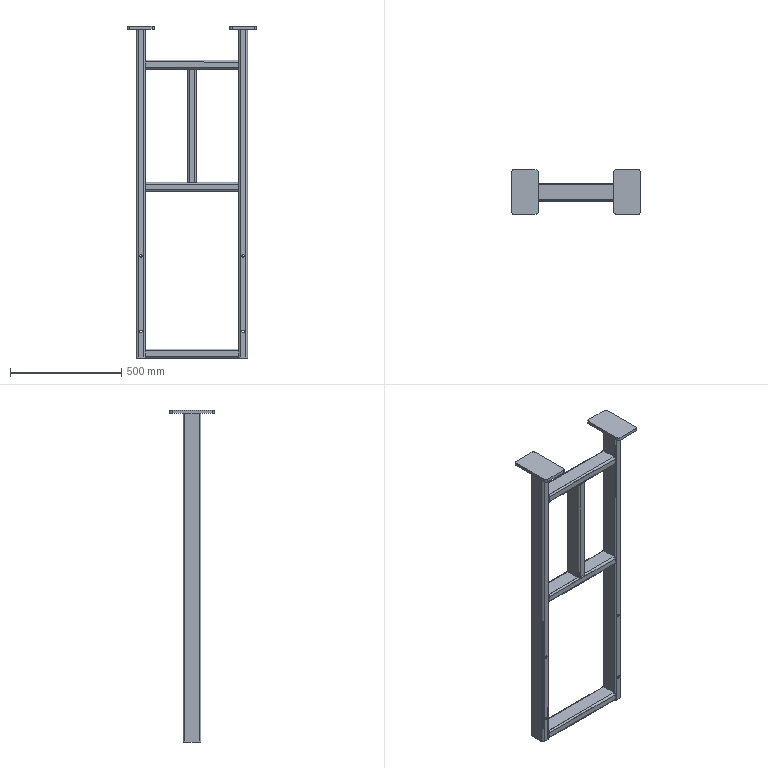Part | SolidWorks | features MirrorSolid 3, WeldMemberFeat 3, 3DProfileFeature 2, WeldCornerFeat 2, Cut 1, Fillet 1, ICE 1, LPattern 1, MoveCopyBody 1, WeldmentFeature 1 | 8 solids | 144 faces | box 580 x 200 x 1494 mm | volume 4709165 mm3 | plane 72 | cylinder 72 | commonest cylinder face diameters 8 x24 16 x24 12 x16 20 x8